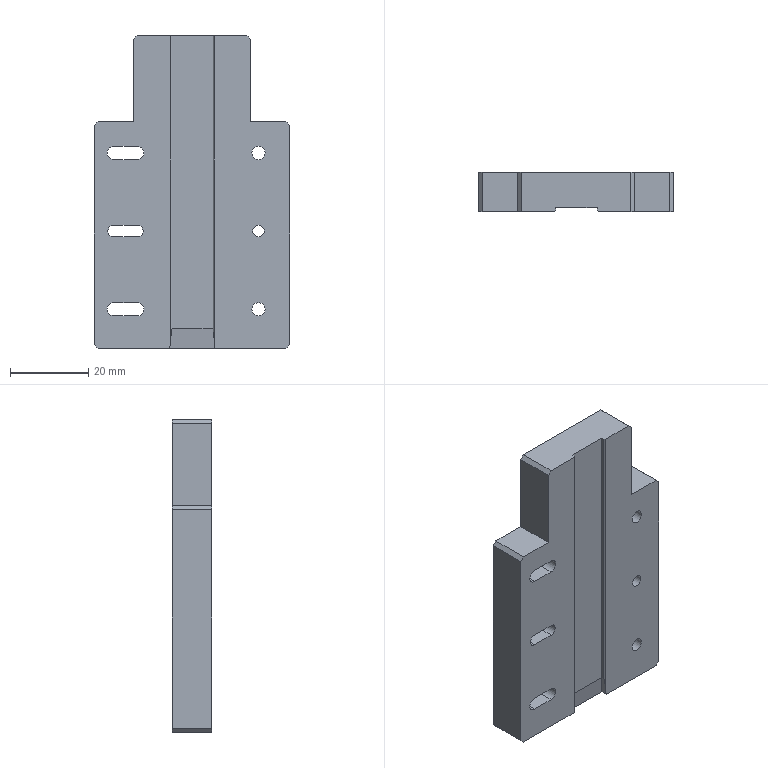Part | 1 solid | 54 faces | box 50 x 10 x 80 mm | volume 32938 mm3 | plane 39 | cylinder 15 | commonest cylinder face diameters 3.4 x6 6.5 x6 3 x3